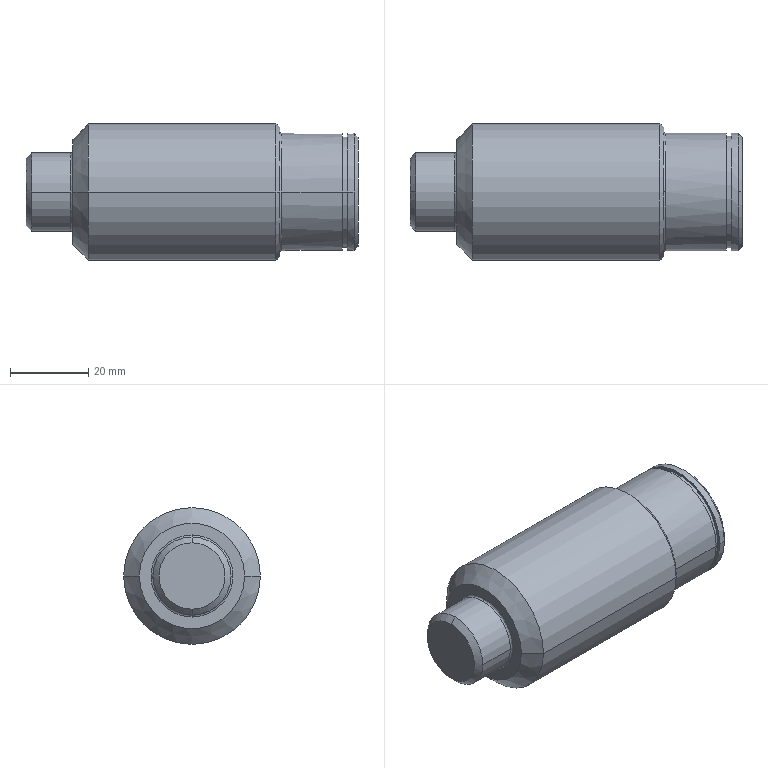Part | SolidWorks | features BaseBody 1 | 1 solid | 28 faces | box 85 x 35 x 35 mm | volume 67829 mm3 | cylinder 10 | cone 8 | plane 6 | spline 4 | commonest cylinder face diameters 30 x4 20 x2 28.6 x2 35 x2
STEP:
#1=CARTESIAN_POINT('',(23.,0.,-15.));
#2=VERTEX_POINT('',#1);
#3=CARTESIAN_POINT('',(23.,15.,0.));
#4=VERTEX_POINT('',#3);
#5=CARTESIAN_POINT('',(23.,0.,0.));
#6=DIRECTION('',(1.,0.,0.));
#7=DIRECTION('',(0.,0.,1.));
#8=AXIS2_PLACEMENT_3D('',#5,#6,#7);
#9=CIRCLE('',#8,15.);
#10=EDGE_CURVE('',#2,#4,#9,.T.);
#11=ORIENTED_EDGE('',*,*,#10,.F.);
#12=CARTESIAN_POINT('',(22.5,0.,-15.5));
#13=VERTEX_POINT('',#12);
#14=CARTESIAN_POINT('',(23.,0.,-15.5));
#15=DIRECTION('',(0.,-1.,0.));
#16=DIRECTION('',(0.,0.,-1.));
#17=AXIS2_PLACEMENT_3D('',#14,#15,#16);
#18=CIRCLE('',#17,0.5);
#19=EDGE_CURVE('',#2,#13,#18,.T.);
#20=ORIENTED_EDGE('',*,*,#19,.T.);
#21=CARTESIAN_POINT('',(22.5,0.,15.5));
#22=VERTEX_POINT('',#21);
#23=CARTESIAN_POINT('',(22.5,0.,15.5));
#24=CARTESIAN_POINT('',(22.5,0.4739,15.5));
#25=CARTESIAN_POINT('',(22.5,1.182,15.468));
#26=CARTESIAN_POINT('',(22.5,2.003,15.373));
#27=CARTESIAN_POINT('',(22.5,2.412,15.312));
#28=CARTESIAN_POINT('',(22.5,2.616,15.278));
#29=CARTESIAN_POINT('',(22.5,2.704,15.262));
#30=CARTESIAN_POINT('',(22.5,2.762,15.252));
#31=CARTESIAN_POINT('',(22.5,2.79,15.247));
#32=CARTESIAN_POINT('',(22.5,3.315,15.15));
#33=CARTESIAN_POINT('',(22.5,4.046,14.978));
#34=CARTESIAN_POINT('',(22.5,4.881,14.715));
#35=CARTESIAN_POINT('',(22.5,5.295,14.569));
#36=CARTESIAN_POINT('',(22.5,5.501,14.491));
#37=CARTESIAN_POINT('',(22.5,5.588,14.458));
#38=CARTESIAN_POINT('',(22.5,5.647,14.435));
#39=CARTESIAN_POINT('',(22.5,5.675,14.424));
#40=CARTESIAN_POINT('',(22.5,6.192,14.219));
#41=CARTESIAN_POINT('',(22.5,6.905,13.895));
#42=CARTESIAN_POINT('',(22.5,7.704,13.455));
#43=CARTESIAN_POINT('',(22.5,8.095,13.219));
#44=CARTESIAN_POINT('',(22.5,8.262,13.115));
#45=CARTESIAN_POINT('',(22.5,8.372,13.045));
#46=CARTESIAN_POINT('',(22.5,8.426,13.01));
#47=CARTESIAN_POINT('',(22.5,9.377,12.388));
#48=CARTESIAN_POINT('',(22.5,10.204,11.717));
#49=CARTESIAN_POINT('',(22.5,11.338,10.582));
#50=CARTESIAN_POINT('',(22.5,11.874,9.989));
#51=CARTESIAN_POINT('',(22.5,12.442,9.25));
#52=CARTESIAN_POINT('',(22.5,12.712,8.87));
#53=CARTESIAN_POINT('',(22.5,12.825,8.704));
#54=CARTESIAN_POINT('',(22.5,12.9,8.593));
#55=CARTESIAN_POINT('',(22.5,12.938,8.537));
#56=CARTESIAN_POINT('',(22.5,13.26,8.043));
#57=CARTESIAN_POINT('',(22.5,13.655,7.368));
#58=CARTESIAN_POINT('',(22.5,14.054,6.547));
#59=CARTESIAN_POINT('',(22.5,14.238,6.129));
#60=CARTESIAN_POINT('',(22.5,14.326,5.918));
#61=CARTESIAN_POINT('',(22.5,14.363,5.827));
#62=CARTESIAN_POINT('',(22.5,14.388,5.766));
#63=CARTESIAN_POINT('',(22.5,14.4,5.735));
#64=CARTESIAN_POINT('',(22.5,14.597,5.238));
#65=CARTESIAN_POINT('',(22.5,14.839,4.527));
#66=CARTESIAN_POINT('',(22.5,15.061,3.68));
#67=CARTESIAN_POINT('',(22.5,15.156,3.252));
#68=CARTESIAN_POINT('',(22.5,15.2,3.036));
#69=CARTESIAN_POINT('',(22.5,15.218,2.944));
#70=CARTESIAN_POINT('',(22.5,15.23,2.882));
#71=CARTESIAN_POINT('',(22.5,15.236,2.85));
#72=CARTESIAN_POINT('',(22.5,15.414,1.889));
#73=CARTESIAN_POINT('',(22.5,15.5,0.9477));
#74=CARTESIAN_POINT('',(22.5,15.5,-0.4739));
#75=CARTESIAN_POINT('',(22.5,15.468,-1.182));
#76=CARTESIAN_POINT('',(22.5,15.373,-2.003));
#77=CARTESIAN_POINT('',(22.5,15.312,-2.412));
#78=CARTESIAN_POINT('',(22.5,15.278,-2.616));
#79=CARTESIAN_POINT('',(22.5,15.262,-2.704));
#80=CARTESIAN_POINT('',(22.5,15.252,-2.762));
#81=CARTESIAN_POINT('',(22.5,15.247,-2.79));
#82=CARTESIAN_POINT('',(22.5,15.15,-3.315));
#83=CARTESIAN_POINT('',(22.5,14.978,-4.046));
#84=CARTESIAN_POINT('',(22.5,14.715,-4.881));
#85=CARTESIAN_POINT('',(22.5,14.569,-5.295));
#86=CARTESIAN_POINT('',(22.5,14.491,-5.501));
#87=CARTESIAN_POINT('',(22.5,14.458,-5.588));
#88=CARTESIAN_POINT('',(22.5,14.435,-5.647));
#89=CARTESIAN_POINT('',(22.5,14.424,-5.675));
#90=CARTESIAN_POINT('',(22.5,14.219,-6.192));
#91=CARTESIAN_POINT('',(22.5,13.895,-6.905));
#92=CARTESIAN_POINT('',(22.5,13.455,-7.704));
#93=CARTESIAN_POINT('',(22.5,13.219,-8.095));
#94=CARTESIAN_POINT('',(22.5,13.115,-8.262));
#95=CARTESIAN_POINT('',(22.5,13.045,-8.372));
#96=CARTESIAN_POINT('',(22.5,13.01,-8.426));
#97=CARTESIAN_POINT('',(22.5,12.388,-9.377));
#98=CARTESIAN_POINT('',(22.5,11.717,-10.204));
#99=CARTESIAN_POINT('',(22.5,10.582,-11.338));
#100=CARTESIAN_POINT('',(22.5,9.989,-11.874));
#101=CARTESIAN_POINT('',(22.5,9.25,-12.442));
#102=CARTESIAN_POINT('',(22.5,8.87,-12.712));
#103=CARTESIAN_POINT('',(22.5,8.704,-12.825));
#104=CARTESIAN_POINT('',(22.5,8.593,-12.9));
#105=CARTESIAN_POINT('',(22.5,8.537,-12.938));
#106=CARTESIAN_POINT('',(22.5,8.043,-13.26));
#107=CARTESIAN_POINT('',(22.5,7.368,-13.655));
#108=CARTESIAN_POINT('',(22.5,6.547,-14.054));
#109=CARTESIAN_POINT('',(22.5,6.129,-14.238));
#110=CARTESIAN_POINT('',(22.5,5.918,-14.326));
#111=CARTESIAN_POINT('',(22.5,5.827,-14.363));
#112=CARTESIAN_POINT('',(22.5,5.766,-14.388));
#113=CARTESIAN_POINT('',(22.5,5.735,-14.4));
#114=CARTESIAN_POINT('',(22.5,5.238,-14.597));
#115=CARTESIAN_POINT('',(22.5,4.527,-14.839));
#116=CARTESIAN_POINT('',(22.5,3.68,-15.061));
#117=CARTESIAN_POINT('',(22.5,3.252,-15.156));
#118=CARTESIAN_POINT('',(22.5,3.036,-15.2));
#119=CARTESIAN_POINT('',(22.5,2.944,-15.218));
#120=CARTESIAN_POINT('',(22.5,2.882,-15.23));
#121=CARTESIAN_POINT('',(22.5,2.85,-15.236));
#122=CARTESIAN_POINT('',(22.5,1.889,-15.414));
#123=CARTESIAN_POINT('',(22.5,0.9477,-15.5));
#124=CARTESIAN_POINT('',(22.5,0.,-15.5));
#125=B_SPLINE_CURVE_WITH_KNOTS('',3,(#23,#24,#25,#26,#27,#28,#29,#30,#31,#32,#33,#34,#35,#36,#37,#38,#39,#40,#41,#42,#43,#44,#45,#46,#47,#48,#49,#50,#51,#52,#53,#54,#55,#56,#57,#58,#59,#60,#61,#62,#63,#64,#65,#66,#67,#68,#69,#70,#71,#72,#73,#74,#75,#76,#77,#78,#79,#80,#81,#82,#83,#84,#85,#86,#87,#88,#89,#90,#91,#92,#93,#94,#95,#96,#97,#98,#99,#100,#101,#102,#103,#104,#105,#106,#107,#108,#109,#110,#111,#112,#113,#114,#115,#116,#117,#118,#119,#120,#121,#122,#123,#124),.UNSPECIFIED.,.F.,.F.,(4,1,1,1,1,2,2,1,1,1,1,2,2,1,1,1,2,2,2,1,1,1,2,2,1,1,1,1,2,2,1,1,1,1,2,2,2,1,1,1,1,2,2,1,1,1,1,2,2,1,1,1,2,2,2,1,1,1,2,2,1,1,1,1,2,2,1,1,1,1,2,2,4),(0.25,0.2656,0.2734,0.2773,0.2793,0.2803,0.2812,0.2969,0.3047,0.3086,0.3105,0.3115,0.3125,0.3281,0.3359,0.3398,0.3418,0.3437,0.375,0.3906,0.3984,0.4023,0.4043,0.4062,0.4219,0.4297,0.4336,0.4355,0.4365,0.4375,0.4531,0.4609,0.4648,0.4668,0.4678,0.4687,0.5,0.5156,0.5234,0.5273,0.5293,0.5303,0.5312,0.5469,0.5547,0.5586,0.5605,0.5615,0.5625,0.5781,0.5859,0.5898,0.5918,0.5937,0.625,0.6406,0.6484,0.6523,0.6543,0.6562,0.6719,0.6797,0.6836,0.6855,0.6865,0.6875,0.7031,0.7109,0.7148,0.7168,0.7178,0.7187,0.75),.UNSPECIFIED.);
#126=EDGE_CURVE('',#22,#13,#125,.T.);
#127=ORIENTED_EDGE('',*,*,#126,.F.);
#128=CARTESIAN_POINT('',(23.,0.,15.));
#129=VERTEX_POINT('',#128);
#130=CARTESIAN_POINT('',(23.,0.,15.5));
#131=DIRECTION('',(0.,1.,0.));
#132=DIRECTION('',(0.,0.,1.));
#133=AXIS2_PLACEMENT_3D('',#130,#131,#132);
#134=CIRCLE('',#133,0.5);
#135=EDGE_CURVE('',#129,#22,#134,.T.);
#136=ORIENTED_EDGE('',*,*,#135,.F.);
#137=CARTESIAN_POINT('',(23.,0.,0.));
#138=DIRECTION('',(1.,0.,0.));
#139=DIRECTION('',(0.,0.,1.));
#140=AXIS2_PLACEMENT_3D('',#137,#138,#139);
#141=CIRCLE('',#140,15.);
#142=EDGE_CURVE('',#4,#129,#141,.T.);
#143=ORIENTED_EDGE('',*,*,#142,.F.);
#144=EDGE_LOOP('',(#11,#20,#127,#136,#143));
#145=FACE_OUTER_BOUND('',#144,.T.);
#146=CARTESIAN_POINT('',(23.,0.,15.));
#147=CARTESIAN_POINT('',(23.,30.,15.));
#148=CARTESIAN_POINT('',(23.,30.,-15.));
#149=CARTESIAN_POINT('',(23.,0.,-15.));
#150=CARTESIAN_POINT('',(22.707,0.,15.));
#151=CARTESIAN_POINT('',(22.707,30.,15.));
#152=CARTESIAN_POINT('',(22.707,30.,-15.));
#153=CARTESIAN_POINT('',(22.707,0.,-15.));
#154=CARTESIAN_POINT('',(22.5,0.,15.207));
#155=CARTESIAN_POINT('',(22.5,30.414,15.207));
#156=CARTESIAN_POINT('',(22.5,30.414,-15.207));
#157=CARTESIAN_POINT('',(22.5,0.,-15.207));
#158=CARTESIAN_POINT('',(22.5,0.,15.5));
#159=CARTESIAN_POINT('',(22.5,31.,15.5));
#160=CARTESIAN_POINT('',(22.5,31.,-15.5));
#161=CARTESIAN_POINT('',(22.5,0.,-15.5));
#162=(BOUNDED_SURFACE()B_SPLINE_SURFACE(3,3,((#146,#147,#148,#149),(#150,#151,#152,#153),(#154,#155,#156,#157),(#158,#159,#160,#161)),.UNSPECIFIED.,.F.,.F.,.T.)B_SPLINE_SURFACE_WITH_KNOTS((4,4),(4,4),(0.,1.),(0.,1.),.UNSPECIFIED.)GEOMETRIC_REPRESENTATION_ITEM()RATIONAL_B_SPLINE_SURFACE(((1.,0.3333,0.3333,1.),(0.8047,0.2682,0.2682,0.8047),(0.8047,0.2682,0.2682,0.8047),(1.,0.3333,0.3333,1.)))REPRESENTATION_ITEM('')SURFACE());
#163=ADVANCED_FACE('',(#145),#162,.F.);
#164=CARTESIAN_POINT('',(-30.5,0.,-10.5));
#165=VERTEX_POINT('',#164);
#166=CARTESIAN_POINT('',(-30.5,0.,10.5));
#167=VERTEX_POINT('',#166);
#168=CARTESIAN_POINT('',(-30.5,0.,-10.5));
#169=CARTESIAN_POINT('',(-30.5,0.3209,-10.5));
#170=CARTESIAN_POINT('',(-30.5,0.8005,-10.478));
#171=CARTESIAN_POINT('',(-30.5,1.357,-10.414));
#172=CARTESIAN_POINT('',(-30.5,1.634,-10.373));
#173=CARTESIAN_POINT('',(-30.5,1.772,-10.349));
#174=CARTESIAN_POINT('',(-30.5,1.832,-10.339));
#175=CARTESIAN_POINT('',(-30.5,1.871,-10.332));
#176=CARTESIAN_POINT('',(-30.5,1.89,-10.329));
#177=CARTESIAN_POINT('',(-30.5,2.245,-10.263));
#178=CARTESIAN_POINT('',(-30.5,2.741,-10.146));
#179=CARTESIAN_POINT('',(-30.5,3.307,-9.968));
#180=CARTESIAN_POINT('',(-30.5,3.587,-9.869));
#181=CARTESIAN_POINT('',(-30.5,3.706,-9.824));
#182=CARTESIAN_POINT('',(-30.5,3.786,-9.794));
#183=CARTESIAN_POINT('',(-30.5,3.824,-9.779));
#184=CARTESIAN_POINT('',(-30.5,4.195,-9.632));
#185=CARTESIAN_POINT('',(-30.5,4.677,-9.413));
#186=CARTESIAN_POINT('',(-30.5,5.219,-9.114));
#187=CARTESIAN_POINT('',(-30.5,5.446,-8.978));
#188=CARTESIAN_POINT('',(-30.5,5.597,-8.885));
#189=CARTESIAN_POINT('',(-30.5,5.67,-8.838));
#190=CARTESIAN_POINT('',(-30.5,6.352,-8.392));
#191=CARTESIAN_POINT('',(-30.5,6.912,-7.937));
#192=CARTESIAN_POINT('',(-30.5,7.681,-7.168));
#193=CARTESIAN_POINT('',(-30.5,8.043,-6.767));
#194=CARTESIAN_POINT('',(-30.5,8.429,-6.266));
#195=CARTESIAN_POINT('',(-30.5,8.586,-6.046));
#196=CARTESIAN_POINT('',(-30.5,8.688,-5.897));
#197=CARTESIAN_POINT('',(-30.5,8.74,-5.82));
#198=CARTESIAN_POINT('',(-30.5,8.983,-5.449));
#199=CARTESIAN_POINT('',(-30.5,9.25,-4.991));
#200=CARTESIAN_POINT('',(-30.5,9.52,-4.435));
#201=CARTESIAN_POINT('',(-30.5,9.645,-4.152));
#202=CARTESIAN_POINT('',(-30.5,9.696,-4.029));
#203=CARTESIAN_POINT('',(-30.5,9.73,-3.947));
#204=CARTESIAN_POINT('',(-30.5,9.747,-3.905));
#205=CARTESIAN_POINT('',(-30.5,9.888,-3.549));
#206=CARTESIAN_POINT('',(-30.5,10.052,-3.067));
#207=CARTESIAN_POINT('',(-30.5,10.202,-2.493));
#208=CARTESIAN_POINT('',(-30.5,10.267,-2.203));
#209=CARTESIAN_POINT('',(-30.5,10.297,-2.057));
#210=CARTESIAN_POINT('',(-30.5,10.309,-1.994));
#211=CARTESIAN_POINT('',(-30.5,10.317,-1.952));
#212=CARTESIAN_POINT('',(-30.5,10.321,-1.93));
#213=CARTESIAN_POINT('',(-30.5,10.442,-1.279));
#214=CARTESIAN_POINT('',(-30.5,10.5,-0.6419));
#215=CARTESIAN_POINT('',(-30.5,10.5,0.3209));
#216=CARTESIAN_POINT('',(-30.5,10.478,0.8005));
#217=CARTESIAN_POINT('',(-30.5,10.414,1.357));
#218=CARTESIAN_POINT('',(-30.5,10.373,1.634));
#219=CARTESIAN_POINT('',(-30.5,10.349,1.772));
#220=CARTESIAN_POINT('',(-30.5,10.339,1.832));
#221=CARTESIAN_POINT('',(-30.5,10.332,1.871));
#222=CARTESIAN_POINT('',(-30.5,10.329,1.89));
#223=CARTESIAN_POINT('',(-30.5,10.263,2.245));
#224=CARTESIAN_POINT('',(-30.5,10.146,2.741));
#225=CARTESIAN_POINT('',(-30.5,9.968,3.307));
#226=CARTESIAN_POINT('',(-30.5,9.869,3.587));
#227=CARTESIAN_POINT('',(-30.5,9.824,3.706));
#228=CARTESIAN_POINT('',(-30.5,9.794,3.786));
#229=CARTESIAN_POINT('',(-30.5,9.779,3.824));
#230=CARTESIAN_POINT('',(-30.5,9.632,4.195));
#231=CARTESIAN_POINT('',(-30.5,9.413,4.677));
#232=CARTESIAN_POINT('',(-30.5,9.114,5.219));
#233=CARTESIAN_POINT('',(-30.5,8.978,5.446));
#234=CARTESIAN_POINT('',(-30.5,8.885,5.597));
#235=CARTESIAN_POINT('',(-30.5,8.838,5.67));
#236=CARTESIAN_POINT('',(-30.5,8.392,6.352));
#237=CARTESIAN_POINT('',(-30.5,7.937,6.912));
#238=CARTESIAN_POINT('',(-30.5,7.168,7.681));
#239=CARTESIAN_POINT('',(-30.5,6.767,8.043));
#240=CARTESIAN_POINT('',(-30.5,6.266,8.429));
#241=CARTESIAN_POINT('',(-30.5,6.046,8.586));
#242=CARTESIAN_POINT('',(-30.5,5.897,8.688));
#243=CARTESIAN_POINT('',(-30.5,5.82,8.74));
#244=CARTESIAN_POINT('',(-30.5,5.449,8.983));
#245=CARTESIAN_POINT('',(-30.5,4.991,9.25));
#246=CARTESIAN_POINT('',(-30.5,4.435,9.52));
#247=CARTESIAN_POINT('',(-30.5,4.152,9.645));
#248=CARTESIAN_POINT('',(-30.5,4.029,9.696));
#249=CARTESIAN_POINT('',(-30.5,3.947,9.73));
#250=CARTESIAN_POINT('',(-30.5,3.905,9.747));
#251=CARTESIAN_POINT('',(-30.5,3.549,9.888));
#252=CARTESIAN_POINT('',(-30.5,3.067,10.052));
#253=CARTESIAN_POINT('',(-30.5,2.493,10.202));
#254=CARTESIAN_POINT('',(-30.5,2.203,10.267));
#255=CARTESIAN_POINT('',(-30.5,2.057,10.297));
#256=CARTESIAN_POINT('',(-30.5,1.994,10.309));
#257=CARTESIAN_POINT('',(-30.5,1.952,10.317));
#258=CARTESIAN_POINT('',(-30.5,1.93,10.321));
#259=CARTESIAN_POINT('',(-30.5,1.279,10.442));
#260=CARTESIAN_POINT('',(-30.5,0.6419,10.5));
#261=CARTESIAN_POINT('',(-30.5,0.,10.5));
#262=B_SPLINE_CURVE_WITH_KNOTS('',3,(#168,#169,#170,#171,#172,#173,#174,#175,#176,#177,#178,#179,#180,#181,#182,#183,#184,#185,#186,#187,#188,#189,#190,#191,#192,#193,#194,#195,#196,#197,#198,#199,#200,#201,#202,#203,#204,#205,#206,#207,#208,#209,#210,#211,#212,#213,#214,#215,#216,#217,#218,#219,#220,#221,#222,#223,#224,#225,#226,#227,#228,#229,#230,#231,#232,#233,#234,#235,#236,#237,#238,#239,#240,#241,#242,#243,#244,#245,#246,#247,#248,#249,#250,#251,#252,#253,#254,#255,#256,#257,#258,#259,#260,#261),.UNSPECIFIED.,.F.,.F.,(4,1,1,1,1,2,2,1,1,1,2,2,1,1,2,2,2,1,1,2,2,1,1,1,2,2,1,1,1,1,2,2,2,1,1,1,1,2,2,1,1,1,2,2,1,1,2,2,2,1,1,2,2,1,1,1,2,2,1,1,1,1,2,2,4),(0.25,0.2656,0.2734,0.2773,0.2793,0.2803,0.2812,0.2969,0.3047,0.3086,0.3105,0.3125,0.3281,0.3359,0.3398,0.3437,0.375,0.3906,0.3984,0.4023,0.4062,0.4219,0.4297,0.4336,0.4355,0.4375,0.4531,0.4609,0.4648,0.4668,0.4678,0.4687,0.5,0.5156,0.5234,0.5273,0.5293,0.5303,0.5313,0.5469,0.5547,0.5586,0.5605,0.5625,0.5781,0.5859,0.5898,0.5938,0.625,0.6406,0.6484,0.6523,0.6563,0.6719,0.6797,0.6836,0.6855,0.6875,0.7031,0.7109,0.7148,0.7168,0.7178,0.7188,0.75),.UNSPECIFIED.);
#263=EDGE_CURVE('',#165,#167,#262,.T.);
#264=ORIENTED_EDGE('',*,*,#263,.F.);
#265=CARTESIAN_POINT('',(-31.,0.,-10.));
#266=VERTEX_POINT('',#265);
#267=CARTESIAN_POINT('',(-31.,0.,-10.5));
#268=DIRECTION('',(0.,-1.,0.));
#269=DIRECTION('',(0.,0.,-1.));
#270=AXIS2_PLACEMENT_3D('',#267,#268,#269);
#271=CIRCLE('',#270,0.5);
#272=EDGE_CURVE('',#165,#266,#271,.T.);
#273=ORIENTED_EDGE('',*,*,#272,.T.);
#274=CARTESIAN_POINT('',(-31.,10.,0.));
#275=VERTEX_POINT('',#274);
#276=CARTESIAN_POINT('',(-31.,0.,0.));
#277=DIRECTION('',(-1.,0.,0.));
#278=DIRECTION('',(0.,0.,1.));
#279=AXIS2_PLACEMENT_3D('',#276,#277,#278);
#280=CIRCLE('',#279,10.);
#281=EDGE_CURVE('',#275,#266,#280,.T.);
#282=ORIENTED_EDGE('',*,*,#281,.F.);
#283=CARTESIAN_POINT('',(-31.,0.,10.));
#284=VERTEX_POINT('',#283);
#285=CARTESIAN_POINT('',(-31.,0.,0.));
#286=DIRECTION('',(-1.,0.,0.));
#287=DIRECTION('',(0.,0.,1.));
#288=AXIS2_PLACEMENT_3D('',#285,#286,#287);
#289=CIRCLE('',#288,10.);
#290=EDGE_CURVE('',#284,#275,#289,.T.);
#291=ORIENTED_EDGE('',*,*,#290,.F.);
#292=CARTESIAN_POINT('',(-31.,0.,10.5));
#293=DIRECTION('',(0.,1.,0.));
#294=DIRECTION('',(0.,0.,1.));
#295=AXIS2_PLACEMENT_3D('',#292,#293,#294);
#296=CIRCLE('',#295,0.5);
#297=EDGE_CURVE('',#167,#284,#296,.T.);
#298=ORIENTED_EDGE('',*,*,#297,.F.);
#299=EDGE_LOOP('',(#264,#273,#282,#291,#298));
#300=FACE_OUTER_BOUND('',#299,.T.);
#301=CARTESIAN_POINT('',(-30.5,0.,10.5));
#302=CARTESIAN_POINT('',(-30.5,21.,10.5));
#303=CARTESIAN_POINT('',(-30.5,21.,-10.5));
#304=CARTESIAN_POINT('',(-30.5,0.,-10.5));
#305=CARTESIAN_POINT('',(-30.5,0.,10.207));
#306=CARTESIAN_POINT('',(-30.5,20.414,10.207));
#307=CARTESIAN_POINT('',(-30.5,20.414,-10.207));
#308=CARTESIAN_POINT('',(-30.5,0.,-10.207));
#309=CARTESIAN_POINT('',(-30.707,0.,10.));
#310=CARTESIAN_POINT('',(-30.707,20.,10.));
#311=CARTESIAN_POINT('',(-30.707,20.,-10.));
#312=CARTESIAN_POINT('',(-30.707,0.,-10.));
#313=CARTESIAN_POINT('',(-31.,0.,10.));
#314=CARTESIAN_POINT('',(-31.,20.,10.));
#315=CARTESIAN_POINT('',(-31.,20.,-10.));
#316=CARTESIAN_POINT('',(-31.,0.,-10.));
#317=(BOUNDED_SURFACE()B_SPLINE_SURFACE(3,3,((#301,#302,#303,#304),(#305,#306,#307,#308),(#309,#310,#311,#312),(#313,#314,#315,#316)),.UNSPECIFIED.,.F.,.F.,.T.)B_SPLINE_SURFACE_WITH_KNOTS((4,4),(4,4),(0.,1.),(0.,1.),.UNSPECIFIED.)GEOMETRIC_REPRESENTATION_ITEM()RATIONAL_B_SPLINE_SURFACE(((1.,0.3333,0.3333,1.),(0.8047,0.2682,0.2682,0.8047),(0.8047,0.2682,0.2682,0.8047),(1.,0.3333,0.3333,1.)))REPRESENTATION_ITEM('')SURFACE());
#318=ADVANCED_FACE('',(#300),#317,.F.);
#319=CARTESIAN_POINT('',(21.5,-17.5,0.));
#320=VERTEX_POINT('',#319);
#321=CARTESIAN_POINT('',(21.5,17.5,0.));
#322=VERTEX_POINT('',#321);
#323=CARTESIAN_POINT('',(21.5,0.,0.));
#324=DIRECTION('',(-1.,0.,0.));
#325=DIRECTION('',(0.,-1.,0.));
#326=AXIS2_PLACEMENT_3D('',#323,#324,#325);
#327=CIRCLE('',#326,17.5);
#328=EDGE_CURVE('',#320,#322,#327,.T.);
#329=ORIENTED_EDGE('',*,*,#328,.T.);
#330=CARTESIAN_POINT('',(-26.5,17.5,0.));
#331=VERTEX_POINT('',#330);
#332=CARTESIAN_POINT('',(-2.5,17.5,0.));
#333=DIRECTION('',(-1.,0.,0.));
#334=VECTOR('',#333,1000.);
#335=LINE('',#332,#334);
#336=EDGE_CURVE('',#322,#331,#335,.T.);
#337=ORIENTED_EDGE('',*,*,#336,.T.);
#338=CARTESIAN_POINT('',(-26.5,-17.5,0.));
#339=VERTEX_POINT('',#338);
#340=CARTESIAN_POINT('',(-26.5,0.,0.));
#341=DIRECTION('',(1.,0.,0.));
#342=DIRECTION('',(0.,-1.,0.));
#343=AXIS2_PLACEMENT_3D('',#340,#341,#342);
#344=CIRCLE('',#343,17.5);
#345=EDGE_CURVE('',#331,#339,#344,.T.);
#346=ORIENTED_EDGE('',*,*,#345,.T.);
#347=CARTESIAN_POINT('',(-2.5,-17.5,0.));
#348=DIRECTION('',(-1.,0.,0.));
#349=VECTOR('',#348,1000.);
#350=LINE('',#347,#349);
#351=EDGE_CURVE('',#320,#339,#350,.T.);
#352=ORIENTED_EDGE('',*,*,#351,.F.);
#353=EDGE_LOOP('',(#329,#337,#346,#352));
#354=FACE_OUTER_BOUND('',#353,.T.);
#355=CARTESIAN_POINT('',(-2.5,0.,0.));
#356=DIRECTION('',(-1.,0.,0.));
#357=DIRECTION('',(0.,-1.,0.));
#358=AXIS2_PLACEMENT_3D('',#355,#356,#357);
#359=CYLINDRICAL_SURFACE('',#358,17.5);
#360=ADVANCED_FACE('',(#354),#359,.T.);
#361=CARTESIAN_POINT('',(22.5,-16.5,0.));
#362=VERTEX_POINT('',#361);
#363=CARTESIAN_POINT('',(22.5,16.5,0.));
#364=VERTEX_POINT('',#363);
#365=CARTESIAN_POINT('',(22.5,0.,0.));
#366=DIRECTION('',(-1.,0.,0.));
#367=DIRECTION('',(0.,-1.,0.));
#368=AXIS2_PLACEMENT_3D('',#365,#366,#367);
#369=CIRCLE('',#368,16.5);
#370=EDGE_CURVE('',#362,#364,#369,.T.);
#371=ORIENTED_EDGE('',*,*,#370,.T.);
#372=CARTESIAN_POINT('',(21.5,17.5,0.));
#373=DIRECTION('',(-0.7071,0.7071,0.));
#374=VECTOR('',#373,1000.);
#375=LINE('',#372,#374);
#376=EDGE_CURVE('',#364,#322,#375,.T.);
#377=ORIENTED_EDGE('',*,*,#376,.T.);
#378=ORIENTED_EDGE('',*,*,#328,.F.);
#379=CARTESIAN_POINT('',(21.5,-17.5,0.));
#380=DIRECTION('',(-0.7071,-0.7071,0.));
#381=VECTOR('',#380,1000.);
#382=LINE('',#379,#381);
#383=EDGE_CURVE('',#362,#320,#382,.T.);
#384=ORIENTED_EDGE('',*,*,#383,.F.);
#385=EDGE_LOOP('',(#371,#377,#378,#384));
#386=FACE_OUTER_BOUND('',#385,.T.);
#387=CARTESIAN_POINT('',(21.5,0.,0.));
#388=DIRECTION('',(-1.,0.,0.));
#389=DIRECTION('',(0.,-1.,0.));
#390=AXIS2_PLACEMENT_3D('',#387,#388,#389);
#391=CONICAL_SURFACE('',#390,17.5,0.7854);
#392=ADVANCED_FACE('',(#386),#391,.T.);
#393=CARTESIAN_POINT('',(-30.5,13.5,0.));
#394=VERTEX_POINT('',#393);
#395=CARTESIAN_POINT('',(-30.5,-13.5,0.));
#396=VERTEX_POINT('',#395);
#397=CARTESIAN_POINT('',(-30.5,0.,0.));
#398=DIRECTION('',(1.,0.,0.));
#399=DIRECTION('',(0.,1.,0.));
#400=AXIS2_PLACEMENT_3D('',#397,#398,#399);
#401=CIRCLE('',#400,13.5);
#402=EDGE_CURVE('',#394,#396,#401,.T.);
#403=ORIENTED_EDGE('',*,*,#402,.T.);
#404=CARTESIAN_POINT('',(-26.5,-17.5,0.));
#405=DIRECTION('',(0.7071,-0.7071,0.));
#406=VECTOR('',#405,1000.);
#407=LINE('',#404,#406);
#408=EDGE_CURVE('',#396,#339,#407,.T.);
#409=ORIENTED_EDGE('',*,*,#408,.T.);
#410=ORIENTED_EDGE('',*,*,#345,.F.);
#411=CARTESIAN_POINT('',(-26.5,17.5,0.));
#412=DIRECTION('',(0.7071,0.7071,0.));
#413=VECTOR('',#412,1000.);
#414=LINE('',#411,#413);
#415=EDGE_CURVE('',#394,#331,#414,.T.);
#416=ORIENTED_EDGE('',*,*,#415,.F.);
#417=EDGE_LOOP('',(#403,#409,#410,#416));
#418=FACE_OUTER_BOUND('',#417,.T.);
#419=CARTESIAN_POINT('',(-26.5,0.,0.));
#420=DIRECTION('',(1.,0.,0.));
#421=DIRECTION('',(0.,1.,0.));
#422=AXIS2_PLACEMENT_3D('',#419,#420,#421);
#423=CONICAL_SURFACE('',#422,17.5,0.7854);
#424=ADVANCED_FACE('',(#418),#423,.T.);
#425=CARTESIAN_POINT('',(38.5,-15.,0.));
#426=VERTEX_POINT('',#425);
#427=CARTESIAN_POINT('',(38.5,15.,0.));
#428=VERTEX_POINT('',#427);
#429=CARTESIAN_POINT('',(38.5,0.,0.));
#430=DIRECTION('',(-1.,0.,0.));
#431=DIRECTION('',(0.,-1.,0.));
#432=AXIS2_PLACEMENT_3D('',#429,#430,#431);
#433=CIRCLE('',#432,15.);
#434=EDGE_CURVE('',#426,#428,#433,.T.);
#435=ORIENTED_EDGE('',*,*,#434,.T.);
#436=CARTESIAN_POINT('',(30.75,15.,0.));
#437=DIRECTION('',(-1.,0.,0.));
#438=VECTOR('',#437,1000.);
#439=LINE('',#436,#438);
#440=EDGE_CURVE('',#428,#4,#439,.T.);
#441=ORIENTED_EDGE('',*,*,#440,.T.);
#442=ORIENTED_EDGE('',*,*,#142,.T.);
#443=CARTESIAN_POINT('',(23.,-15.,0.));
#444=VERTEX_POINT('',#443);
#445=CARTESIAN_POINT('',(23.,0.,0.));
#446=DIRECTION('',(1.,0.,0.));
#447=DIRECTION('',(0.,0.,1.));
#448=AXIS2_PLACEMENT_3D('',#445,#446,#447);
#449=CIRCLE('',#448,15.);
#450=EDGE_CURVE('',#129,#444,#449,.T.);
#451=ORIENTED_EDGE('',*,*,#450,.T.);
#452=CARTESIAN_POINT('',(30.75,-15.,0.));
#453=DIRECTION('',(-1.,0.,0.));
#454=VECTOR('',#453,1000.);
#455=LINE('',#452,#454);
#456=EDGE_CURVE('',#426,#444,#455,.T.);
#457=ORIENTED_EDGE('',*,*,#456,.F.);
#458=EDGE_LOOP('',(#435,#441,#442,#451,#457));
#459=FACE_OUTER_BOUND('',#458,.T.);
#460=CARTESIAN_POINT('',(30.75,0.,0.));
#461=DIRECTION('',(-1.,0.,0.));
#462=DIRECTION('',(0.,-1.,0.));
#463=AXIS2_PLACEMENT_3D('',#460,#461,#462);
#464=CYLINDRICAL_SURFACE('',#463,15.);
#465=ADVANCED_FACE('',(#459),#464,.T.);
#466=CARTESIAN_POINT('',(-31.,-10.,0.));
#467=VERTEX_POINT('',#466);
#468=CARTESIAN_POINT('',(-31.,0.,0.));
#469=DIRECTION('',(-1.,0.,0.));
#470=DIRECTION('',(0.,0.,1.));
#471=AXIS2_PLACEMENT_3D('',#468,#469,#470);
#472=CIRCLE('',#471,10.);
#473=EDGE_CURVE('',#467,#284,#472,.T.);
#474=ORIENTED_EDGE('',*,*,#473,.T.);
#475=ORIENTED_EDGE('',*,*,#290,.T.);
#476=CARTESIAN_POINT('',(-41.,10.,0.));
#477=VERTEX_POINT('',#476);
#478=CARTESIAN_POINT('',(-36.75,10.,0.));
#479=DIRECTION('',(-1.,0.,0.));
#480=VECTOR('',#479,1000.);
#481=LINE('',#478,#480);
#482=EDGE_CURVE('',#275,#477,#481,.T.);
#483=ORIENTED_EDGE('',*,*,#482,.T.);
#484=CARTESIAN_POINT('',(-41.,0.,10.));
#485=VERTEX_POINT('',#484);
#486=CARTESIAN_POINT('',(-41.,0.,0.));
#487=DIRECTION('',(1.,0.,0.));
#488=DIRECTION('',(0.,-1.,0.));
#489=AXIS2_PLACEMENT_3D('',#486,#487,#488);
#490=CIRCLE('',#489,10.);
#491=EDGE_CURVE('',#477,#485,#490,.T.);
#492=ORIENTED_EDGE('',*,*,#491,.T.);
#493=CARTESIAN_POINT('',(-41.,-10.,0.));
#494=VERTEX_POINT('',#493);
#495=CARTESIAN_POINT('',(-41.,0.,0.));
#496=DIRECTION('',(1.,0.,0.));
#497=DIRECTION('',(0.,-1.,0.));
#498=AXIS2_PLACEMENT_3D('',#495,#496,#497);
#499=CIRCLE('',#498,10.);
#500=EDGE_CURVE('',#485,#494,#499,.T.);
#501=ORIENTED_EDGE('',*,*,#500,.T.);
#502=CARTESIAN_POINT('',(-36.75,-10.,0.));
#503=DIRECTION('',(-1.,0.,0.));
#504=VECTOR('',#503,1000.);
#505=LINE('',#502,#504);
#506=EDGE_CURVE('',#467,#494,#505,.T.);
#507=ORIENTED_EDGE('',*,*,#506,.F.);
#508=EDGE_LOOP('',(#474,#475,#483,#492,#501,#507));
#509=FACE_OUTER_BOUND('',#508,.T.);
#510=CARTESIAN_POINT('',(-36.75,0.,0.));
#511=DIRECTION('',(-1.,0.,0.));
#512=DIRECTION('',(0.,-1.,0.));
#513=AXIS2_PLACEMENT_3D('',#510,#511,#512);
#514=CYLINDRICAL_SURFACE('',#513,10.);
#515=ADVANCED_FACE('',(#509),#514,.T.);
#516=CARTESIAN_POINT('',(-42.5,0.,-8.5));
#517=VERTEX_POINT('',#516);
#518=CARTESIAN_POINT('',(-42.5,0.,8.5));
#519=VERTEX_POINT('',#518);
#520=CARTESIAN_POINT('',(-42.5,0.,0.));
#521=DIRECTION('',(1.,0.,0.));
#522=DIRECTION('',(0.,0.,-1.));
#523=AXIS2_PLACEMENT_3D('',#520,#521,#522);
#524=CIRCLE('',#523,8.5);
#525=EDGE_CURVE('',#517,#519,#524,.T.);
#526=ORIENTED_EDGE('',*,*,#525,.T.);
#527=CARTESIAN_POINT('',(-41.,0.,10.));
#528=DIRECTION('',(0.7071,0.,0.7071));
#529=VECTOR('',#528,1000.);
#530=LINE('',#527,#529);
#531=EDGE_CURVE('',#519,#485,#530,.T.);
#532=ORIENTED_EDGE('',*,*,#531,.T.);
#533=ORIENTED_EDGE('',*,*,#491,.F.);
#534=CARTESIAN_POINT('',(-41.,0.,-10.));
#535=VERTEX_POINT('',#534);
#536=CARTESIAN_POINT('',(-41.,0.,0.));
#537=DIRECTION('',(1.,0.,0.));
#538=DIRECTION('',(0.,-1.,0.));
#539=AXIS2_PLACEMENT_3D('',#536,#537,#538);
#540=CIRCLE('',#539,10.);
#541=EDGE_CURVE('',#535,#477,#540,.T.);
#542=ORIENTED_EDGE('',*,*,#541,.F.);
#543=CARTESIAN_POINT('',(-41.,0.,-10.));
#544=DIRECTION('',(0.7071,0.,-0.7071));
#545=VECTOR('',#544,1000.);
#546=LINE('',#543,#545);
#547=EDGE_CURVE('',#517,#535,#546,.T.);
#548=ORIENTED_EDGE('',*,*,#547,.F.);
#549=EDGE_LOOP('',(#526,#532,#533,#542,#548));
#550=FACE_OUTER_BOUND('',#549,.T.);
#551=CARTESIAN_POINT('',(-41.,0.,0.));
#552=DIRECTION('',(1.,0.,0.));
#553=DIRECTION('',(0.,0.,-1.));
#554=AXIS2_PLACEMENT_3D('',#551,#552,#553);
#555=CONICAL_SURFACE('',#554,10.,0.7854);
#556=ADVANCED_FACE('',(#550),#555,.T.);
#557=CARTESIAN_POINT('',(39.8,-14.3,0.));
#558=VERTEX_POINT('',#557);
#559=CARTESIAN_POINT('',(39.8,14.3,0.));
#560=VERTEX_POINT('',#559);
#561=CARTESIAN_POINT('',(39.8,0.,0.));
#562=DIRECTION('',(-1.,0.,0.));
#563=DIRECTION('',(0.,-1.,0.));
#564=AXIS2_PLACEMENT_3D('',#561,#562,#563);
#565=CIRCLE('',#564,14.3);
#566=EDGE_CURVE('',#558,#560,#565,.T.);
#567=ORIENTED_EDGE('',*,*,#566,.T.);
#568=CARTESIAN_POINT('',(38.5,14.3,0.));
#569=VERTEX_POINT('',#568);
#570=CARTESIAN_POINT('',(39.15,14.3,0.));
#571=DIRECTION('',(-1.,0.,0.));
#572=VECTOR('',#571,1000.);
#573=LINE('',#570,#572);
#574=EDGE_CURVE('',#560,#569,#573,.T.);
#575=ORIENTED_EDGE('',*,*,#574,.T.);
#576=CARTESIAN_POINT('',(38.5,-14.3,0.));
#577=VERTEX_POINT('',#576);
#578=CARTESIAN_POINT('',(38.5,0.,0.));
#579=DIRECTION('',(-1.,0.,0.));
#580=DIRECTION('',(0.,-1.,0.));
#581=AXIS2_PLACEMENT_3D('',#578,#579,#580);
#582=CIRCLE('',#581,14.3);
#583=EDGE_CURVE('',#577,#569,#582,.T.);
#584=ORIENTED_EDGE('',*,*,#583,.F.);
#585=CARTESIAN_POINT('',(39.15,-14.3,0.));
#586=DIRECTION('',(-1.,0.,0.));
#587=VECTOR('',#586,1000.);
#588=LINE('',#585,#587);
#589=EDGE_CURVE('',#558,#577,#588,.T.);
#590=ORIENTED_EDGE('',*,*,#589,.F.);
#591=EDGE_LOOP('',(#567,#575,#584,#590));
#592=FACE_OUTER_BOUND('',#591,.T.);
#593=CARTESIAN_POINT('',(39.15,0.,0.));
#594=DIRECTION('',(-1.,0.,0.));
#595=DIRECTION('',(0.,-1.,0.));
#596=AXIS2_PLACEMENT_3D('',#593,#594,#595);
#597=CYLINDRICAL_SURFACE('',#596,14.3);
#598=ADVANCED_FACE('',(#592),#597,.T.);
#599=CARTESIAN_POINT('',(41.5,0.,15.));
#600=VERTEX_POINT('',#599);
#601=CARTESIAN_POINT('',(41.5,15.,0.));
#602=VERTEX_POINT('',#601);
#603=CARTESIAN_POINT('',(41.5,0.,0.));
#604=DIRECTION('',(-1.,0.,0.));
#605=DIRECTION('',(0.,-1.,0.));
#606=AXIS2_PLACEMENT_3D('',#603,#604,#605);
#607=CIRCLE('',#606,15.);
#608=EDGE_CURVE('',#600,#602,#607,.T.);
#609=ORIENTED_EDGE('',*,*,#608,.T.);
#610=CARTESIAN_POINT('',(39.8,15.,0.));
#611=VERTEX_POINT('',#610);
#612=CARTESIAN_POINT('',(40.65,15.,0.));
#613=DIRECTION('',(-1.,0.,0.));
#614=VECTOR('',#613,1000.);
#615=LINE('',#612,#614);
#616=EDGE_CURVE('',#602,#611,#615,.T.);
#617=ORIENTED_EDGE('',*,*,#616,.T.);
#618=CARTESIAN_POINT('',(39.8,-15.,0.));
#619=VERTEX_POINT('',#618);
#620=CARTESIAN_POINT('',(39.8,0.,0.));
#621=DIRECTION('',(-1.,0.,0.));
#622=DIRECTION('',(0.,-1.,0.));
#623=AXIS2_PLACEMENT_3D('',#620,#621,#622);
#624=CIRCLE('',#623,15.);
#625=EDGE_CURVE('',#619,#611,#624,.T.);
#626=ORIENTED_EDGE('',*,*,#625,.F.);
#627=CARTESIAN_POINT('',(41.5,-15.,0.));
#628=VERTEX_POINT('',#627);
#629=CARTESIAN_POINT('',(40.65,-15.,0.));
#630=DIRECTION('',(-1.,0.,0.));
#631=VECTOR('',#630,1000.);
#632=LINE('',#629,#631);
#633=EDGE_CURVE('',#628,#619,#632,.T.);
#634=ORIENTED_EDGE('',*,*,#633,.F.);
#635=CARTESIAN_POINT('',(41.5,0.,0.));
#636=DIRECTION('',(-1.,0.,0.));
#637=DIRECTION('',(0.,-1.,0.));
#638=AXIS2_PLACEMENT_3D('',#635,#636,#637);
#639=CIRCLE('',#638,15.);
#640=EDGE_CURVE('',#628,#600,#639,.T.);
#641=ORIENTED_EDGE('',*,*,#640,.T.);
#642=EDGE_LOOP('',(#609,#617,#626,#634,#641));
#643=FACE_OUTER_BOUND('',#642,.T.);
#644=CARTESIAN_POINT('',(40.65,0.,0.));
#645=DIRECTION('',(-1.,0.,0.));
#646=DIRECTION('',(0.,-1.,0.));
#647=AXIS2_PLACEMENT_3D('',#644,#645,#646);
#648=CYLINDRICAL_SURFACE('',#647,15.);
#649=ADVANCED_FACE('',(#643),#648,.T.);
#650=CARTESIAN_POINT('',(42.5,0.,14.));
#651=VERTEX_POINT('',#650);
#652=CARTESIAN_POINT('',(42.5,0.,-14.));
#653=VERTEX_POINT('',#652);
#654=CARTESIAN_POINT('',(42.5,0.,0.));
#655=DIRECTION('',(-1.,0.,0.));
#656=DIRECTION('',(0.,0.,1.));
#657=AXIS2_PLACEMENT_3D('',#654,#655,#656);
#658=CIRCLE('',#657,14.);
#659=EDGE_CURVE('',#651,#653,#658,.T.);
#660=ORIENTED_EDGE('',*,*,#659,.T.);
#661=CARTESIAN_POINT('',(41.5,0.,-15.));
#662=VERTEX_POINT('',#661);
#663=CARTESIAN_POINT('',(41.5,0.,-15.));
#664=DIRECTION('',(-0.7071,0.,-0.7071));
#665=VECTOR('',#664,1000.);
#666=LINE('',#663,#665);
#667=EDGE_CURVE('',#653,#662,#666,.T.);
#668=ORIENTED_EDGE('',*,*,#667,.T.);
#669=CARTESIAN_POINT('',(41.5,0.,0.));
#670=DIRECTION('',(-1.,0.,0.));
#671=DIRECTION('',(0.,-1.,0.));
#672=AXIS2_PLACEMENT_3D('',#669,#670,#671);
#673=CIRCLE('',#672,15.);
#674=EDGE_CURVE('',#602,#662,#673,.T.);
#675=ORIENTED_EDGE('',*,*,#674,.F.);
#676=ORIENTED_EDGE('',*,*,#608,.F.);
#677=CARTESIAN_POINT('',(41.5,0.,15.));
#678=DIRECTION('',(-0.7071,0.,0.7071));
#679=VECTOR('',#678,1000.);
#680=LINE('',#677,#679);
#681=EDGE_CURVE('',#651,#600,#680,.T.);
#682=ORIENTED_EDGE('',*,*,#681,.F.);
#683=EDGE_LOOP('',(#660,#668,#675,#676,#682));
#684=FACE_OUTER_BOUND('',#683,.T.);
#685=CARTESIAN_POINT('',(41.5,0.,0.));
#686=DIRECTION('',(-1.,0.,0.));
#687=DIRECTION('',(0.,0.,1.));
#688=AXIS2_PLACEMENT_3D('',#685,#686,#687);
#689=CONICAL_SURFACE('',#688,15.,0.7854);
#690=ADVANCED_FACE('',(#684),#689,.T.);
#691=ORIENTED_EDGE('',*,*,#336,.F.);
#692=CARTESIAN_POINT('',(21.5,0.,0.));
#693=DIRECTION('',(-1.,0.,0.));
#694=DIRECTION('',(0.,-1.,0.));
#695=AXIS2_PLACEMENT_3D('',#692,#693,#694);
#696=CIRCLE('',#695,17.5);
#697=EDGE_CURVE('',#322,#320,#696,.T.);
#698=ORIENTED_EDGE('',*,*,#697,.T.);
#699=ORIENTED_EDGE('',*,*,#351,.T.);
#700=CARTESIAN_POINT('',(-26.5,0.,0.));
#701=DIRECTION('',(1.,0.,0.));
#702=DIRECTION('',(0.,-1.,0.));
#703=AXIS2_PLACEMENT_3D('',#700,#701,#702);
#704=CIRCLE('',#703,17.5);
#705=EDGE_CURVE('',#339,#331,#704,.T.);
#706=ORIENTED_EDGE('',*,*,#705,.T.);
#707=EDGE_LOOP('',(#691,#698,#699,#706));
#708=FACE_OUTER_BOUND('',#707,.T.);
#709=CARTESIAN_POINT('',(-2.5,0.,0.));
#710=DIRECTION('',(-1.,0.,0.));
#711=DIRECTION('',(0.,-1.,0.));
#712=AXIS2_PLACEMENT_3D('',#709,#710,#711);
#713=CYLINDRICAL_SURFACE('',#712,17.5);
#714=ADVANCED_FACE('',(#708),#713,.T.);
#715=ORIENTED_EDGE('',*,*,#376,.F.);
#716=CARTESIAN_POINT('',(22.5,0.,0.));
#717=DIRECTION('',(-1.,0.,0.));
#718=DIRECTION('',(0.,-1.,0.));
#719=AXIS2_PLACEMENT_3D('',#716,#717,#718);
#720=CIRCLE('',#719,16.5);
#721=EDGE_CURVE('',#364,#362,#720,.T.);
#722=ORIENTED_EDGE('',*,*,#721,.T.);
#723=ORIENTED_EDGE('',*,*,#383,.T.);
#724=ORIENTED_EDGE('',*,*,#697,.F.);
#725=EDGE_LOOP('',(#715,#722,#723,#724));
#726=FACE_OUTER_BOUND('',#725,.T.);
#727=CARTESIAN_POINT('',(21.5,0.,0.));
#728=DIRECTION('',(-1.,0.,0.));
#729=DIRECTION('',(0.,-1.,0.));
#730=AXIS2_PLACEMENT_3D('',#727,#728,#729);
#731=CONICAL_SURFACE('',#730,17.5,0.7854);
#732=ADVANCED_FACE('',(#726),#731,.T.);
#733=ORIENTED_EDGE('',*,*,#408,.F.);
#734=CARTESIAN_POINT('',(-30.5,0.,0.));
#735=DIRECTION('',(1.,0.,0.));
#736=DIRECTION('',(0.,1.,0.));
#737=AXIS2_PLACEMENT_3D('',#734,#735,#736);
#738=CIRCLE('',#737,13.5);
#739=EDGE_CURVE('',#396,#394,#738,.T.);
#740=ORIENTED_EDGE('',*,*,#739,.T.);
#741=ORIENTED_EDGE('',*,*,#415,.T.);
#742=ORIENTED_EDGE('',*,*,#705,.F.);
#743=EDGE_LOOP('',(#733,#740,#741,#742));
#744=FACE_OUTER_BOUND('',#743,.T.);
#745=CARTESIAN_POINT('',(-26.5,0.,0.));
#746=DIRECTION('',(1.,0.,0.));
#747=DIRECTION('',(0.,1.,0.));
#748=AXIS2_PLACEMENT_3D('',#745,#746,#747);
#749=CONICAL_SURFACE('',#748,17.5,0.7854);
#750=ADVANCED_FACE('',(#744),#749,.T.);
#751=ORIENTED_EDGE('',*,*,#126,.T.);
#752=CARTESIAN_POINT('',(22.5,0.,-15.5));
#753=CARTESIAN_POINT('',(22.5,-0.4739,-15.5));
#754=CARTESIAN_POINT('',(22.5,-1.182,-15.468));
#755=CARTESIAN_POINT('',(22.5,-2.003,-15.373));
#756=CARTESIAN_POINT('',(22.5,-2.412,-15.312));
#757=CARTESIAN_POINT('',(22.5,-2.616,-15.278));
#758=CARTESIAN_POINT('',(22.5,-2.704,-15.262));
#759=CARTESIAN_POINT('',(22.5,-2.762,-15.252));
#760=CARTESIAN_POINT('',(22.5,-2.79,-15.247));
#761=CARTESIAN_POINT('',(22.5,-3.315,-15.15));
#762=CARTESIAN_POINT('',(22.5,-4.046,-14.978));
#763=CARTESIAN_POINT('',(22.5,-4.881,-14.715));
#764=CARTESIAN_POINT('',(22.5,-5.295,-14.569));
#765=CARTESIAN_POINT('',(22.5,-5.501,-14.491));
#766=CARTESIAN_POINT('',(22.5,-5.588,-14.458));
#767=CARTESIAN_POINT('',(22.5,-5.647,-14.435));
#768=CARTESIAN_POINT('',(22.5,-5.675,-14.424));
#769=CARTESIAN_POINT('',(22.5,-6.192,-14.219));
#770=CARTESIAN_POINT('',(22.5,-6.905,-13.895));
#771=CARTESIAN_POINT('',(22.5,-7.704,-13.455));
#772=CARTESIAN_POINT('',(22.5,-8.095,-13.219));
#773=CARTESIAN_POINT('',(22.5,-8.262,-13.115));
#774=CARTESIAN_POINT('',(22.5,-8.372,-13.045));
#775=CARTESIAN_POINT('',(22.5,-8.426,-13.01));
#776=CARTESIAN_POINT('',(22.5,-9.377,-12.388));
#777=CARTESIAN_POINT('',(22.5,-10.204,-11.717));
#778=CARTESIAN_POINT('',(22.5,-11.338,-10.582));
#779=CARTESIAN_POINT('',(22.5,-11.874,-9.989));
#780=CARTESIAN_POINT('',(22.5,-12.442,-9.25));
#781=CARTESIAN_POINT('',(22.5,-12.712,-8.87));
#782=CARTESIAN_POINT('',(22.5,-12.825,-8.704));
#783=CARTESIAN_POINT('',(22.5,-12.9,-8.593));
#784=CARTESIAN_POINT('',(22.5,-12.938,-8.537));
#785=CARTESIAN_POINT('',(22.5,-13.26,-8.043));
#786=CARTESIAN_POINT('',(22.5,-13.655,-7.368));
#787=CARTESIAN_POINT('',(22.5,-14.054,-6.547));
#788=CARTESIAN_POINT('',(22.5,-14.238,-6.129));
#789=CARTESIAN_POINT('',(22.5,-14.326,-5.918));
#790=CARTESIAN_POINT('',(22.5,-14.363,-5.827));
#791=CARTESIAN_POINT('',(22.5,-14.388,-5.766));
#792=CARTESIAN_POINT('',(22.5,-14.4,-5.735));
#793=CARTESIAN_POINT('',(22.5,-14.597,-5.238));
#794=CARTESIAN_POINT('',(22.5,-14.839,-4.527));
#795=CARTESIAN_POINT('',(22.5,-15.061,-3.68));
#796=CARTESIAN_POINT('',(22.5,-15.156,-3.252));
#797=CARTESIAN_POINT('',(22.5,-15.2,-3.036));
#798=CARTESIAN_POINT('',(22.5,-15.218,-2.944));
#799=CARTESIAN_POINT('',(22.5,-15.23,-2.882));
#800=CARTESIAN_POINT('',(22.5,-15.236,-2.85));
#801=CARTESIAN_POINT('',(22.5,-15.414,-1.888));
#802=CARTESIAN_POINT('',(22.5,-15.5,-0.9479));
#803=CARTESIAN_POINT('',(22.5,-15.5,0.4739));
#804=CARTESIAN_POINT('',(22.5,-15.478,0.9462));
#805=CARTESIAN_POINT('',(22.5,-15.414,1.651));
#806=CARTESIAN_POINT('',(22.5,-15.373,2.003));
#807=CARTESIAN_POINT('',(22.5,-15.312,2.412));
#808=CARTESIAN_POINT('',(22.5,-15.278,2.616));
#809=CARTESIAN_POINT('',(22.5,-15.262,2.704));
#810=CARTESIAN_POINT('',(22.5,-15.252,2.762));
#811=CARTESIAN_POINT('',(22.5,-15.247,2.79));
#812=CARTESIAN_POINT('',(22.5,-15.15,3.315));
#813=CARTESIAN_POINT('',(22.5,-14.978,4.046));
#814=CARTESIAN_POINT('',(22.5,-14.715,4.881));
#815=CARTESIAN_POINT('',(22.5,-14.569,5.295));
#816=CARTESIAN_POINT('',(22.5,-14.491,5.501));
#817=CARTESIAN_POINT('',(22.5,-14.458,5.588));
#818=CARTESIAN_POINT('',(22.5,-14.435,5.647));
#819=CARTESIAN_POINT('',(22.5,-14.424,5.675));
#820=CARTESIAN_POINT('',(22.5,-14.219,6.192));
#821=CARTESIAN_POINT('',(22.5,-13.895,6.905));
#822=CARTESIAN_POINT('',(22.5,-13.455,7.704));
#823=CARTESIAN_POINT('',(22.5,-13.219,8.095));
#824=CARTESIAN_POINT('',(22.5,-13.115,8.262));
#825=CARTESIAN_POINT('',(22.5,-13.045,8.372));
#826=CARTESIAN_POINT('',(22.5,-13.01,8.426));
#827=CARTESIAN_POINT('',(22.5,-12.388,9.377));
#828=CARTESIAN_POINT('',(22.5,-11.717,10.204));
#829=CARTESIAN_POINT('',(22.5,-10.582,11.338));
#830=CARTESIAN_POINT('',(22.5,-9.989,11.874));
#831=CARTESIAN_POINT('',(22.5,-9.25,12.442));
#832=CARTESIAN_POINT('',(22.5,-8.87,12.712));
#833=CARTESIAN_POINT('',(22.5,-8.704,12.825));
#834=CARTESIAN_POINT('',(22.5,-8.593,12.9));
#835=CARTESIAN_POINT('',(22.5,-8.537,12.938));
#836=CARTESIAN_POINT('',(22.5,-8.043,13.26));
#837=CARTESIAN_POINT('',(22.5,-7.368,13.655));
#838=CARTESIAN_POINT('',(22.5,-6.547,14.054));
#839=CARTESIAN_POINT('',(22.5,-6.129,14.238));
#840=CARTESIAN_POINT('',(22.5,-5.918,14.326));
#841=CARTESIAN_POINT('',(22.5,-5.827,14.363));
#842=CARTESIAN_POINT('',(22.5,-5.766,14.388));
#843=CARTESIAN_POINT('',(22.5,-5.735,14.4));
#844=CARTESIAN_POINT('',(22.5,-5.238,14.597));
#845=CARTESIAN_POINT('',(22.5,-4.527,14.839));
#846=CARTESIAN_POINT('',(22.5,-3.68,15.061));
#847=CARTESIAN_POINT('',(22.5,-3.252,15.156));
#848=CARTESIAN_POINT('',(22.5,-3.036,15.2));
#849=CARTESIAN_POINT('',(22.5,-2.944,15.218));
#850=CARTESIAN_POINT('',(22.5,-2.882,15.23));
#851=CARTESIAN_POINT('',(22.5,-2.85,15.236));
#852=CARTESIAN_POINT('',(22.5,-1.889,15.414));
#853=CARTESIAN_POINT('',(22.5,-0.9477,15.5));
#854=CARTESIAN_POINT('',(22.5,0.,15.5));
#855=B_SPLINE_CURVE_WITH_KNOTS('',3,(#752,#753,#754,#755,#756,#757,#758,#759,#760,#761,#762,#763,#764,#765,#766,#767,#768,#769,#770,#771,#772,#773,#774,#775,#776,#777,#778,#779,#780,#781,#782,#783,#784,#785,#786,#787,#788,#789,#790,#791,#792,#793,#794,#795,#796,#797,#798,#799,#800,#801,#802,#803,#804,#805,#806,#807,#808,#809,#810,#811,#812,#813,#814,#815,#816,#817,#818,#819,#820,#821,#822,#823,#824,#825,#826,#827,#828,#829,#830,#831,#832,#833,#834,#835,#836,#837,#838,#839,#840,#841,#842,#843,#844,#845,#846,#847,#848,#849,#850,#851,#852,#853,#854),.UNSPECIFIED.,.F.,.F.,(4,1,1,1,1,2,2,1,1,1,1,2,2,1,1,1,2,2,2,1,1,1,2,2,1,1,1,1,2,2,1,1,1,1,2,2,2,2,1,1,1,2,2,1,1,1,1,2,2,1,1,1,2,2,2,1,1,1,2,2,1,1,1,1,2,2,1,1,1,1,2,2,4),(0.75,0.7656,0.7734,0.7773,0.7793,0.7803,0.7813,0.7969,0.8047,0.8086,0.8105,0.8115,0.8125,0.8281,0.8359,0.8398,0.8418,0.8438,0.875,0.8906,0.8984,0.9023,0.9043,0.9063,0.9219,0.9297,0.9336,0.9355,0.9365,0.9375,0.9531,0.9609,0.9648,0.9668,0.9678,0.9688,1.,1.016,1.023,1.027,1.029,1.03,1.031,1.047,1.055,1.059,1.061,1.062,1.063,1.078,1.086,1.09,1.092,1.094,1.125,1.141,1.148,1.152,1.154,1.156,1.172,1.18,1.184,1.186,1.187,1.188,1.203,1.211,1.215,1.217,1.218,1.219,1.25),.UNSPECIFIED.);
#856=EDGE_CURVE('',#13,#22,#855,.T.);
#857=ORIENTED_EDGE('',*,*,#856,.T.);
#858=EDGE_LOOP('',(#751,#857));
#859=FACE_BOUND('',#858,.T.);
#860=ORIENTED_EDGE('',*,*,#370,.F.);
#861=ORIENTED_EDGE('',*,*,#721,.F.);
#862=EDGE_LOOP('',(#860,#861));
#863=FACE_OUTER_BOUND('',#862,.T.);
#864=CARTESIAN_POINT('',(22.5,-16.5,0.));
#865=DIRECTION('',(1.,0.,0.));
#866=DIRECTION('',(0.,1.,0.));
#867=AXIS2_PLACEMENT_3D('',#864,#865,#866);
#868=PLANE('',#867);
#869=ADVANCED_FACE('',(#859,#863),#868,.T.);
#870=CARTESIAN_POINT('',(-30.5,0.,10.5));
#871=CARTESIAN_POINT('',(-30.5,-0.3209,10.5));
#872=CARTESIAN_POINT('',(-30.5,-0.8005,10.478));
#873=CARTESIAN_POINT('',(-30.5,-1.357,10.414));
#874=CARTESIAN_POINT('',(-30.5,-1.634,10.373));
#875=CARTESIAN_POINT('',(-30.5,-1.772,10.349));
#876=CARTESIAN_POINT('',(-30.5,-1.832,10.339));
#877=CARTESIAN_POINT('',(-30.5,-1.871,10.332));
#878=CARTESIAN_POINT('',(-30.5,-1.89,10.329));
#879=CARTESIAN_POINT('',(-30.5,-2.245,10.263));
#880=CARTESIAN_POINT('',(-30.5,-2.741,10.146));
#881=CARTESIAN_POINT('',(-30.5,-3.307,9.968));
#882=CARTESIAN_POINT('',(-30.5,-3.587,9.869));
#883=CARTESIAN_POINT('',(-30.5,-3.706,9.824));
#884=CARTESIAN_POINT('',(-30.5,-3.786,9.794));
#885=CARTESIAN_POINT('',(-30.5,-3.824,9.779));
#886=CARTESIAN_POINT('',(-30.5,-4.195,9.632));
#887=CARTESIAN_POINT('',(-30.5,-4.677,9.413));
#888=CARTESIAN_POINT('',(-30.5,-5.219,9.114));
#889=CARTESIAN_POINT('',(-30.5,-5.446,8.978));
#890=CARTESIAN_POINT('',(-30.5,-5.597,8.885));
#891=CARTESIAN_POINT('',(-30.5,-5.67,8.838));
#892=CARTESIAN_POINT('',(-30.5,-6.352,8.392));
#893=CARTESIAN_POINT('',(-30.5,-6.912,7.937));
#894=CARTESIAN_POINT('',(-30.5,-7.681,7.168));
#895=CARTESIAN_POINT('',(-30.5,-8.043,6.767));
#896=CARTESIAN_POINT('',(-30.5,-8.429,6.266));
#897=CARTESIAN_POINT('',(-30.5,-8.586,6.046));
#898=CARTESIAN_POINT('',(-30.5,-8.688,5.897));
#899=CARTESIAN_POINT('',(-30.5,-8.74,5.82));
#900=CARTESIAN_POINT('',(-30.5,-8.983,5.449));
#901=CARTESIAN_POINT('',(-30.5,-9.25,4.991));
#902=CARTESIAN_POINT('',(-30.5,-9.52,4.435));
#903=CARTESIAN_POINT('',(-30.5,-9.645,4.152));
#904=CARTESIAN_POINT('',(-30.5,-9.696,4.029));
#905=CARTESIAN_POINT('',(-30.5,-9.73,3.947));
#906=CARTESIAN_POINT('',(-30.5,-9.747,3.905));
#907=CARTESIAN_POINT('',(-30.5,-9.888,3.549));
#908=CARTESIAN_POINT('',(-30.5,-10.052,3.067));
#909=CARTESIAN_POINT('',(-30.5,-10.202,2.493));
#910=CARTESIAN_POINT('',(-30.5,-10.267,2.203));
#911=CARTESIAN_POINT('',(-30.5,-10.297,2.057));
#912=CARTESIAN_POINT('',(-30.5,-10.309,1.994));
#913=CARTESIAN_POINT('',(-30.5,-10.317,1.952));
#914=CARTESIAN_POINT('',(-30.5,-10.321,1.93));
#915=CARTESIAN_POINT('',(-30.5,-10.442,1.279));
#916=CARTESIAN_POINT('',(-30.5,-10.5,0.6421));
#917=CARTESIAN_POINT('',(-30.5,-10.5,-0.321));
#918=CARTESIAN_POINT('',(-30.5,-10.485,-0.641));
#919=CARTESIAN_POINT('',(-30.5,-10.442,-1.119));
#920=CARTESIAN_POINT('',(-30.5,-10.414,-1.357));
#921=CARTESIAN_POINT('',(-30.5,-10.373,-1.634));
#922=CARTESIAN_POINT('',(-30.5,-10.349,-1.772));
#923=CARTESIAN_POINT('',(-30.5,-10.339,-1.832));
#924=CARTESIAN_POINT('',(-30.5,-10.332,-1.871));
#925=CARTESIAN_POINT('',(-30.5,-10.329,-1.89));
#926=CARTESIAN_POINT('',(-30.5,-10.263,-2.245));
#927=CARTESIAN_POINT('',(-30.5,-10.146,-2.741));
#928=CARTESIAN_POINT('',(-30.5,-9.968,-3.307));
#929=CARTESIAN_POINT('',(-30.5,-9.869,-3.587));
#930=CARTESIAN_POINT('',(-30.5,-9.824,-3.706));
#931=CARTESIAN_POINT('',(-30.5,-9.794,-3.786));
#932=CARTESIAN_POINT('',(-30.5,-9.779,-3.824));
#933=CARTESIAN_POINT('',(-30.5,-9.632,-4.195));
#934=CARTESIAN_POINT('',(-30.5,-9.413,-4.677));
#935=CARTESIAN_POINT('',(-30.5,-9.114,-5.219));
#936=CARTESIAN_POINT('',(-30.5,-8.978,-5.446));
#937=CARTESIAN_POINT('',(-30.5,-8.885,-5.597));
#938=CARTESIAN_POINT('',(-30.5,-8.838,-5.67));
#939=CARTESIAN_POINT('',(-30.5,-8.392,-6.352));
#940=CARTESIAN_POINT('',(-30.5,-7.937,-6.912));
#941=CARTESIAN_POINT('',(-30.5,-7.168,-7.681));
#942=CARTESIAN_POINT('',(-30.5,-6.767,-8.043));
#943=CARTESIAN_POINT('',(-30.5,-6.266,-8.429));
#944=CARTESIAN_POINT('',(-30.5,-6.046,-8.586));
#945=CARTESIAN_POINT('',(-30.5,-5.897,-8.688));
#946=CARTESIAN_POINT('',(-30.5,-5.82,-8.74));
#947=CARTESIAN_POINT('',(-30.5,-5.449,-8.983));
#948=CARTESIAN_POINT('',(-30.5,-4.991,-9.25));
#949=CARTESIAN_POINT('',(-30.5,-4.435,-9.52));
#950=CARTESIAN_POINT('',(-30.5,-4.152,-9.645));
#951=CARTESIAN_POINT('',(-30.5,-4.029,-9.696));
#952=CARTESIAN_POINT('',(-30.5,-3.947,-9.73));
#953=CARTESIAN_POINT('',(-30.5,-3.905,-9.747));
#954=CARTESIAN_POINT('',(-30.5,-3.549,-9.888));
#955=CARTESIAN_POINT('',(-30.5,-3.067,-10.052));
#956=CARTESIAN_POINT('',(-30.5,-2.493,-10.202));
#957=CARTESIAN_POINT('',(-30.5,-2.203,-10.267));
#958=CARTESIAN_POINT('',(-30.5,-2.057,-10.297));
#959=CARTESIAN_POINT('',(-30.5,-1.994,-10.309));
#960=CARTESIAN_POINT('',(-30.5,-1.952,-10.317));
#961=CARTESIAN_POINT('',(-30.5,-1.93,-10.321));
#962=CARTESIAN_POINT('',(-30.5,-1.279,-10.442));
#963=CARTESIAN_POINT('',(-30.5,-0.6419,-10.5));
#964=CARTESIAN_POINT('',(-30.5,0.,-10.5));
#965=B_SPLINE_CURVE_WITH_KNOTS('',3,(#870,#871,#872,#873,#874,#875,#876,#877,#878,#879,#880,#881,#882,#883,#884,#885,#886,#887,#888,#889,#890,#891,#892,#893,#894,#895,#896,#897,#898,#899,#900,#901,#902,#903,#904,#905,#906,#907,#908,#909,#910,#911,#912,#913,#914,#915,#916,#917,#918,#919,#920,#921,#922,#923,#924,#925,#926,#927,#928,#929,#930,#931,#932,#933,#934,#935,#936,#937,#938,#939,#940,#941,#942,#943,#944,#945,#946,#947,#948,#949,#950,#951,#952,#953,#954,#955,#956,#957,#958,#959,#960,#961,#962,#963,#964),.UNSPECIFIED.,.F.,.F.,(4,1,1,1,1,2,2,1,1,1,2,2,1,1,2,2,2,1,1,2,2,1,1,1,2,2,1,1,1,1,2,2,2,2,1,1,1,2,2,1,1,1,2,2,1,1,2,2,2,1,1,2,2,1,1,1,2,2,1,1,1,1,2,2,4),(0.75,0.7656,0.7734,0.7773,0.7793,0.7803,0.7812,0.7969,0.8047,0.8086,0.8105,0.8125,0.8281,0.8359,0.8398,0.8437,0.875,0.8906,0.8984,0.9023,0.9062,0.9219,0.9297,0.9336,0.9355,0.9375,0.9531,0.9609,0.9648,0.9668,0.9678,0.9687,1.,1.016,1.023,1.027,1.029,1.03,1.031,1.047,1.055,1.059,1.061,1.062,1.078,1.086,1.09,1.094,1.125,1.141,1.148,1.152,1.156,1.172,1.18,1.184,1.186,1.187,1.203,1.211,1.215,1.217,1.218,1.219,1.25),.UNSPECIFIED.);
#966=EDGE_CURVE('',#167,#165,#965,.T.);
#967=ORIENTED_EDGE('',*,*,#966,.T.);
#968=ORIENTED_EDGE('',*,*,#263,.T.);
#969=EDGE_LOOP('',(#967,#968));
#970=FACE_BOUND('',#969,.T.);
#971=ORIENTED_EDGE('',*,*,#402,.F.);
#972=ORIENTED_EDGE('',*,*,#739,.F.);
#973=EDGE_LOOP('',(#971,#972));
#974=FACE_OUTER_BOUND('',#973,.T.);
#975=CARTESIAN_POINT('',(-30.5,-10.5,0.));
#976=DIRECTION('',(-1.,0.,0.));
#977=DIRECTION('',(0.,-1.,0.));
#978=AXIS2_PLACEMENT_3D('',#975,#976,#977);
#979=PLANE('',#978);
#980=ADVANCED_FACE('',(#970,#974),#979,.T.);
#981=ORIENTED_EDGE('',*,*,#19,.F.);
#982=CARTESIAN_POINT('',(23.,0.,0.));
#983=DIRECTION('',(1.,0.,0.));
#984=DIRECTION('',(0.,0.,1.));
#985=AXIS2_PLACEMENT_3D('',#982,#983,#984);
#986=CIRCLE('',#985,15.);
#987=EDGE_CURVE('',#444,#2,#986,.T.);
#988=ORIENTED_EDGE('',*,*,#987,.F.);
#989=ORIENTED_EDGE('',*,*,#450,.F.);
#990=ORIENTED_EDGE('',*,*,#135,.T.);
#991=ORIENTED_EDGE('',*,*,#856,.F.);
#992=EDGE_LOOP('',(#981,#988,#989,#990,#991));
#993=FACE_OUTER_BOUND('',#992,.T.);
#994=CARTESIAN_POINT('',(23.,0.,-15.));
#995=CARTESIAN_POINT('',(23.,-30.,-15.));
#996=CARTESIAN_POINT('',(23.,-30.,15.));
#997=CARTESIAN_POINT('',(23.,0.,15.));
#998=CARTESIAN_POINT('',(22.707,0.,-15.));
#999=CARTESIAN_POINT('',(22.707,-30.,-15.));
#1000=CARTESIAN_POINT('',(22.707,-30.,15.));
#1001=CARTESIAN_POINT('',(22.707,0.,15.));
#1002=CARTESIAN_POINT('',(22.5,0.,-15.207));
#1003=CARTESIAN_POINT('',(22.5,-30.414,-15.207));
#1004=CARTESIAN_POINT('',(22.5,-30.414,15.207));
#1005=CARTESIAN_POINT('',(22.5,0.,15.207));
#1006=CARTESIAN_POINT('',(22.5,0.,-15.5));
#1007=CARTESIAN_POINT('',(22.5,-31.,-15.5));
#1008=CARTESIAN_POINT('',(22.5,-31.,15.5));
#1009=CARTESIAN_POINT('',(22.5,0.,15.5));
#1010=(BOUNDED_SURFACE()B_SPLINE_SURFACE(3,3,((#994,#995,#996,#997),(#998,#999,#1000,#1001),(#1002,#1003,#1004,#1005),(#1006,#1007,#1008,#1009)),.UNSPECIFIED.,.F.,.F.,.F.)B_SPLINE_SURFACE_WITH_KNOTS((4,4),(4,4),(0.,1.),(0.,1.),.UNSPECIFIED.)GEOMETRIC_REPRESENTATION_ITEM()RATIONAL_B_SPLINE_SURFACE(((1.,0.3333,0.3333,1.),(0.8047,0.2682,0.2682,0.8047),(0.8047,0.2682,0.2682,0.8047),(1.,0.3333,0.3333,1.)))REPRESENTATION_ITEM('')SURFACE());
#1011=ADVANCED_FACE('',(#993),#1010,.F.);
#1012=ORIENTED_EDGE('',*,*,#272,.F.);
#1013=ORIENTED_EDGE('',*,*,#966,.F.);
#1014=ORIENTED_EDGE('',*,*,#297,.T.);
#1015=ORIENTED_EDGE('',*,*,#473,.F.);
#1016=CARTESIAN_POINT('',(-31.,0.,0.));
#1017=DIRECTION('',(-1.,0.,0.));
#1018=DIRECTION('',(0.,0.,1.));
#1019=AXIS2_PLACEMENT_3D('',#1016,#1017,#1018);
#1020=CIRCLE('',#1019,10.);
#1021=EDGE_CURVE('',#266,#467,#1020,.T.);
#1022=ORIENTED_EDGE('',*,*,#1021,.F.);
#1023=EDGE_LOOP('',(#1012,#1013,#1014,#1015,#1022));
#1024=FACE_OUTER_BOUND('',#1023,.T.);
#1025=CARTESIAN_POINT('',(-30.5,0.,-10.5));
#1026=CARTESIAN_POINT('',(-30.5,-21.,-10.5));
#1027=CARTESIAN_POINT('',(-30.5,-21.,10.5));
#1028=CARTESIAN_POINT('',(-30.5,0.,10.5));
#1029=CARTESIAN_POINT('',(-30.5,0.,-10.207));
#1030=CARTESIAN_POINT('',(-30.5,-20.414,-10.207));
#1031=CARTESIAN_POINT('',(-30.5,-20.414,10.207));
#1032=CARTESIAN_POINT('',(-30.5,0.,10.207));
#1033=CARTESIAN_POINT('',(-30.707,0.,-10.));
#1034=CARTESIAN_POINT('',(-30.707,-20.,-10.));
#1035=CARTESIAN_POINT('',(-30.707,-20.,10.));
#1036=CARTESIAN_POINT('',(-30.707,0.,10.));
#1037=CARTESIAN_POINT('',(-31.,0.,-10.));
#1038=CARTESIAN_POINT('',(-31.,-20.,-10.));
#1039=CARTESIAN_POINT('',(-31.,-20.,10.));
#1040=CARTESIAN_POINT('',(-31.,0.,10.));
#1041=(BOUNDED_SURFACE()B_SPLINE_SURFACE(3,3,((#1025,#1026,#1027,#1028),(#1029,#1030,#1031,#1032),(#1033,#1034,#1035,#1036),(#1037,#1038,#1039,#1040)),.UNSPECIFIED.,.F.,.F.,.F.)B_SPLINE_SURFACE_WITH_KNOTS((4,4),(4,4),(0.,1.),(0.,1.),.UNSPECIFIED.)GEOMETRIC_REPRESENTATION_ITEM()RATIONAL_B_SPLINE_SURFACE(((1.,0.3333,0.3333,1.),(0.8047,0.2682,0.2682,0.8047),(0.8047,0.2682,0.2682,0.8047),(1.,0.3333,0.3333,1.)))REPRESENTATION_ITEM('')SURFACE());
#1042=ADVANCED_FACE('',(#1024),#1041,.F.);
#1043=ORIENTED_EDGE('',*,*,#440,.F.);
#1044=CARTESIAN_POINT('',(38.5,0.,0.));
#1045=DIRECTION('',(-1.,0.,0.));
#1046=DIRECTION('',(0.,-1.,0.));
#1047=AXIS2_PLACEMENT_3D('',#1044,#1045,#1046);
#1048=CIRCLE('',#1047,15.);
#1049=EDGE_CURVE('',#428,#426,#1048,.T.);
#1050=ORIENTED_EDGE('',*,*,#1049,.T.);
#1051=ORIENTED_EDGE('',*,*,#456,.T.);
#1052=ORIENTED_EDGE('',*,*,#987,.T.);
#1053=ORIENTED_EDGE('',*,*,#10,.T.);
#1054=EDGE_LOOP('',(#1043,#1050,#1051,#1052,#1053));
#1055=FACE_OUTER_BOUND('',#1054,.T.);
#1056=CARTESIAN_POINT('',(30.75,0.,0.));
#1057=DIRECTION('',(-1.,0.,0.));
#1058=DIRECTION('',(0.,-1.,0.));
#1059=AXIS2_PLACEMENT_3D('',#1056,#1057,#1058);
#1060=CYLINDRICAL_SURFACE('',#1059,15.);
#1061=ADVANCED_FACE('',(#1055),#1060,.T.);
#1062=ORIENTED_EDGE('',*,*,#482,.F.);
#1063=ORIENTED_EDGE('',*,*,#281,.T.);
#1064=ORIENTED_EDGE('',*,*,#1021,.T.);
#1065=ORIENTED_EDGE('',*,*,#506,.T.);
#1066=CARTESIAN_POINT('',(-41.,0.,0.));
#1067=DIRECTION('',(1.,0.,0.));
#1068=DIRECTION('',(0.,-1.,0.));
#1069=AXIS2_PLACEMENT_3D('',#1066,#1067,#1068);
#1070=CIRCLE('',#1069,10.);
#1071=EDGE_CURVE('',#494,#535,#1070,.T.);
#1072=ORIENTED_EDGE('',*,*,#1071,.T.);
#1073=ORIENTED_EDGE('',*,*,#541,.T.);
#1074=EDGE_LOOP('',(#1062,#1063,#1064,#1065,#1072,#1073));
#1075=FACE_OUTER_BOUND('',#1074,.T.);
#1076=CARTESIAN_POINT('',(-36.75,0.,0.));
#1077=DIRECTION('',(-1.,0.,0.));
#1078=DIRECTION('',(0.,-1.,0.));
#1079=AXIS2_PLACEMENT_3D('',#1076,#1077,#1078);
#1080=CYLINDRICAL_SURFACE('',#1079,10.);
#1081=ADVANCED_FACE('',(#1075),#1080,.T.);
#1082=ORIENTED_EDGE('',*,*,#583,.T.);
#1083=CARTESIAN_POINT('',(38.5,0.,0.));
#1084=DIRECTION('',(-1.,0.,0.));
#1085=DIRECTION('',(0.,-1.,0.));
#1086=AXIS2_PLACEMENT_3D('',#1083,#1084,#1085);
#1087=CIRCLE('',#1086,14.3);
#1088=EDGE_CURVE('',#569,#577,#1087,.T.);
#1089=ORIENTED_EDGE('',*,*,#1088,.T.);
#1090=EDGE_LOOP('',(#1082,#1089));
#1091=FACE_BOUND('',#1090,.T.);
#1092=ORIENTED_EDGE('',*,*,#434,.F.);
#1093=ORIENTED_EDGE('',*,*,#1049,.F.);
#1094=EDGE_LOOP('',(#1092,#1093));
#1095=FACE_OUTER_BOUND('',#1094,.T.);
#1096=CARTESIAN_POINT('',(38.5,-15.,0.));
#1097=DIRECTION('',(1.,0.,0.));
#1098=DIRECTION('',(0.,1.,0.));
#1099=AXIS2_PLACEMENT_3D('',#1096,#1097,#1098);
#1100=PLANE('',#1099);
#1101=ADVANCED_FACE('',(#1091,#1095),#1100,.T.);
#1102=ORIENTED_EDGE('',*,*,#531,.F.);
#1103=CARTESIAN_POINT('',(-42.5,0.,0.));
#1104=DIRECTION('',(1.,0.,0.));
#1105=DIRECTION('',(0.,0.,-1.));
#1106=AXIS2_PLACEMENT_3D('',#1103,#1104,#1105);
#1107=CIRCLE('',#1106,8.5);
#1108=EDGE_CURVE('',#519,#517,#1107,.T.);
#1109=ORIENTED_EDGE('',*,*,#1108,.T.);
#1110=ORIENTED_EDGE('',*,*,#547,.T.);
#1111=ORIENTED_EDGE('',*,*,#1071,.F.);
#1112=ORIENTED_EDGE('',*,*,#500,.F.);
#1113=EDGE_LOOP('',(#1102,#1109,#1110,#1111,#1112));
#1114=FACE_OUTER_BOUND('',#1113,.T.);
#1115=CARTESIAN_POINT('',(-41.,0.,0.));
#1116=DIRECTION('',(1.,0.,0.));
#1117=DIRECTION('',(0.,0.,-1.));
#1118=AXIS2_PLACEMENT_3D('',#1115,#1116,#1117);
#1119=CONICAL_SURFACE('',#1118,10.,0.7854);
#1120=ADVANCED_FACE('',(#1114),#1119,.T.);
#1121=ORIENTED_EDGE('',*,*,#574,.F.);
#1122=CARTESIAN_POINT('',(39.8,0.,0.));
#1123=DIRECTION('',(-1.,0.,0.));
#1124=DIRECTION('',(0.,-1.,0.));
#1125=AXIS2_PLACEMENT_3D('',#1122,#1123,#1124);
#1126=CIRCLE('',#1125,14.3);
#1127=EDGE_CURVE('',#560,#558,#1126,.T.);
#1128=ORIENTED_EDGE('',*,*,#1127,.T.);
#1129=ORIENTED_EDGE('',*,*,#589,.T.);
#1130=ORIENTED_EDGE('',*,*,#1088,.F.);
#1131=EDGE_LOOP('',(#1121,#1128,#1129,#1130));
#1132=FACE_OUTER_BOUND('',#1131,.T.);
#1133=CARTESIAN_POINT('',(39.15,0.,0.));
#1134=DIRECTION('',(-1.,0.,0.));
#1135=DIRECTION('',(0.,-1.,0.));
#1136=AXIS2_PLACEMENT_3D('',#1133,#1134,#1135);
#1137=CYLINDRICAL_SURFACE('',#1136,14.3);
#1138=ADVANCED_FACE('',(#1132),#1137,.T.);
#1139=ORIENTED_EDGE('',*,*,#525,.F.);
#1140=ORIENTED_EDGE('',*,*,#1108,.F.);
#1141=EDGE_LOOP('',(#1139,#1140));
#1142=FACE_OUTER_BOUND('',#1141,.T.);
#1143=CARTESIAN_POINT('',(-42.5,0.,0.));
#1144=DIRECTION('',(-1.,0.,0.));
#1145=DIRECTION('',(0.,-1.,0.));
#1146=AXIS2_PLACEMENT_3D('',#1143,#1144,#1145);
#1147=PLANE('',#1146);
#1148=ADVANCED_FACE('',(#1142),#1147,.T.);
#1149=ORIENTED_EDGE('',*,*,#566,.F.);
#1150=ORIENTED_EDGE('',*,*,#1127,.F.);
#1151=EDGE_LOOP('',(#1149,#1150));
#1152=FACE_BOUND('',#1151,.T.);
#1153=ORIENTED_EDGE('',*,*,#625,.T.);
#1154=CARTESIAN_POINT('',(39.8,0.,0.));
#1155=DIRECTION('',(-1.,0.,0.));
#1156=DIRECTION('',(0.,-1.,0.));
#1157=AXIS2_PLACEMENT_3D('',#1154,#1155,#1156);
#1158=CIRCLE('',#1157,15.);
#1159=EDGE_CURVE('',#611,#619,#1158,.T.);
#1160=ORIENTED_EDGE('',*,*,#1159,.T.);
#1161=EDGE_LOOP('',(#1153,#1160));
#1162=FACE_OUTER_BOUND('',#1161,.T.);
#1163=CARTESIAN_POINT('',(39.8,-14.3,0.));
#1164=DIRECTION('',(-1.,0.,0.));
#1165=DIRECTION('',(0.,-1.,0.));
#1166=AXIS2_PLACEMENT_3D('',#1163,#1164,#1165);
#1167=PLANE('',#1166);
#1168=ADVANCED_FACE('',(#1152,#1162),#1167,.T.);
#1169=ORIENTED_EDGE('',*,*,#616,.F.);
#1170=ORIENTED_EDGE('',*,*,#674,.T.);
#1171=CARTESIAN_POINT('',(41.5,0.,0.));
#1172=DIRECTION('',(-1.,0.,0.));
#1173=DIRECTION('',(0.,-1.,0.));
#1174=AXIS2_PLACEMENT_3D('',#1171,#1172,#1173);
#1175=CIRCLE('',#1174,15.);
#1176=EDGE_CURVE('',#662,#628,#1175,.T.);
#1177=ORIENTED_EDGE('',*,*,#1176,.T.);
#1178=ORIENTED_EDGE('',*,*,#633,.T.);
#1179=ORIENTED_EDGE('',*,*,#1159,.F.);
#1180=EDGE_LOOP('',(#1169,#1170,#1177,#1178,#1179));
#1181=FACE_OUTER_BOUND('',#1180,.T.);
#1182=CARTESIAN_POINT('',(40.65,0.,0.));
#1183=DIRECTION('',(-1.,0.,0.));
#1184=DIRECTION('',(0.,-1.,0.));
#1185=AXIS2_PLACEMENT_3D('',#1182,#1183,#1184);
#1186=CYLINDRICAL_SURFACE('',#1185,15.);
#1187=ADVANCED_FACE('',(#1181),#1186,.T.);
#1188=ORIENTED_EDGE('',*,*,#667,.F.);
#1189=CARTESIAN_POINT('',(42.5,0.,0.));
#1190=DIRECTION('',(-1.,0.,0.));
#1191=DIRECTION('',(0.,0.,1.));
#1192=AXIS2_PLACEMENT_3D('',#1189,#1190,#1191);
#1193=CIRCLE('',#1192,14.);
#1194=EDGE_CURVE('',#653,#651,#1193,.T.);
#1195=ORIENTED_EDGE('',*,*,#1194,.T.);
#1196=ORIENTED_EDGE('',*,*,#681,.T.);
#1197=ORIENTED_EDGE('',*,*,#640,.F.);
#1198=ORIENTED_EDGE('',*,*,#1176,.F.);
#1199=EDGE_LOOP('',(#1188,#1195,#1196,#1197,#1198));
#1200=FACE_OUTER_BOUND('',#1199,.T.);
#1201=CARTESIAN_POINT('',(41.5,0.,0.));
#1202=DIRECTION('',(-1.,0.,0.));
#1203=DIRECTION('',(0.,0.,1.));
#1204=AXIS2_PLACEMENT_3D('',#1201,#1202,#1203);
#1205=CONICAL_SURFACE('',#1204,15.,0.7854);
#1206=ADVANCED_FACE('',(#1200),#1205,.T.);
#1207=ORIENTED_EDGE('',*,*,#659,.F.);
#1208=ORIENTED_EDGE('',*,*,#1194,.F.);
#1209=EDGE_LOOP('',(#1207,#1208));
#1210=FACE_OUTER_BOUND('',#1209,.T.);
#1211=CARTESIAN_POINT('',(42.5,-14.,0.));
#1212=DIRECTION('',(1.,0.,0.));
#1213=DIRECTION('',(0.,1.,0.));
#1214=AXIS2_PLACEMENT_3D('',#1211,#1212,#1213);
#1215=PLANE('',#1214);
#1216=ADVANCED_FACE('',(#1210),#1215,.T.);
#1217=CLOSED_SHELL('',(#163,#318,#360,#392,#424,#465,#515,#556,#598,#649,#690,#714,#732,#750,#869,#980,#1011,#1042,#1061,#1081,#1101,#1120,#1138,#1148,#1168,#1187,#1206,#1216));
#1218=MANIFOLD_SOLID_BREP('',#1217);
#1219=CARTESIAN_POINT('',(0.,0.,0.));
#1220=DIRECTION('',(0.,0.,1.));
#1221=DIRECTION('',(1.,0.,0.));
#1222=AXIS2_PLACEMENT_3D('',#1219,#1220,#1221);
#1223=(LENGTH_UNIT()NAMED_UNIT(*)SI_UNIT(.MILLI.,.METRE.));
#1224=UNCERTAINTY_MEASURE_WITH_UNIT(LENGTH_MEASURE(0.00001),#1223,'','');
#1225=(NAMED_UNIT(*)PLANE_ANGLE_UNIT()SI_UNIT($,.RADIAN.));
#1226=(NAMED_UNIT(*)SI_UNIT($,.STERADIAN.)SOLID_ANGLE_UNIT());
#1227=(GEOMETRIC_REPRESENTATION_CONTEXT(3)GLOBAL_UNCERTAINTY_ASSIGNED_CONTEXT((#1224))GLOBAL_UNIT_ASSIGNED_CONTEXT((#1223,#1225,#1226))REPRESENTATION_CONTEXT('',''));
#1228=ADVANCED_BREP_SHAPE_REPRESENTATION('',(#1218,#1222),#1227);